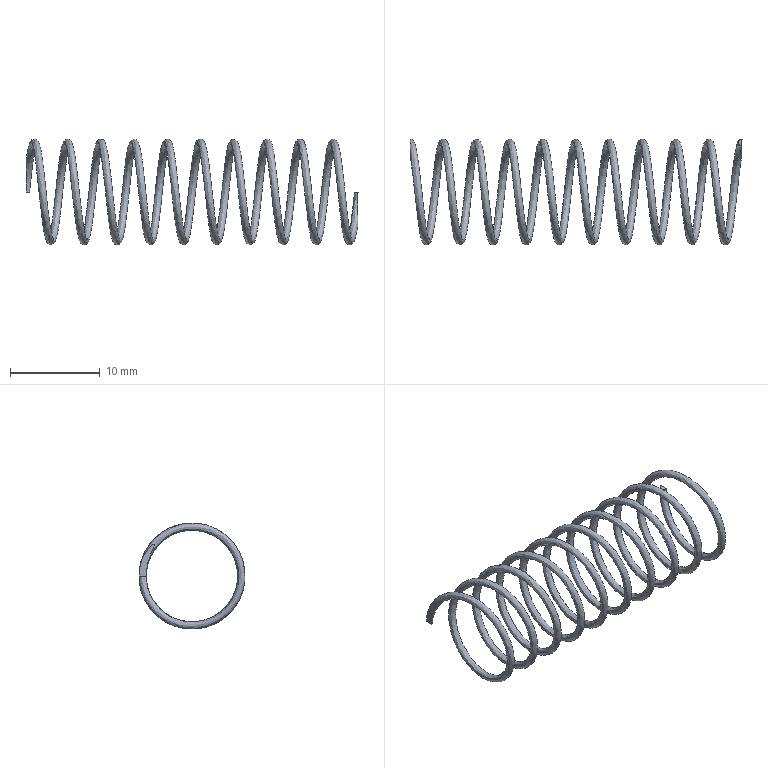Part | NX | features BREP 1, DATUM_CSYS 1 | 1 solid | 5 faces | box 37 x 11.8 x 11.8 mm | volume 173.342 mm3 | plane 4 | spline 1
STEP:
#1=CARTESIAN_POINT('',(0.,5.9,8.));
#2=VERTEX_POINT('',#1);
#3=CARTESIAN_POINT('',(0.,5.1,8.));
#4=VERTEX_POINT('',#3);
#5=CARTESIAN_POINT('',(0.,5.9,8.));
#6=DIRECTION('',(0.,-1.,0.));
#7=VECTOR('',#6,1000.);
#8=LINE('',#5,#7);
#9=EDGE_CURVE('',#2,#4,#8,.T.);
#10=ORIENTED_EDGE('',*,*,#9,.F.);
#11=CARTESIAN_POINT('',(0.4,5.5,8.));
#12=VERTEX_POINT('',#11);
#13=CARTESIAN_POINT('',(0.,5.5,8.));
#14=DIRECTION('',(0.,0.,-1.));
#15=DIRECTION('',(0.,1.,0.));
#16=AXIS2_PLACEMENT_3D('',#13,#14,#15);
#17=CIRCLE('',#16,0.4);
#18=EDGE_CURVE('',#2,#12,#17,.T.);
#19=ORIENTED_EDGE('',*,*,#18,.T.);
#20=CARTESIAN_POINT('',(0.,5.5,8.));
#21=DIRECTION('',(0.,0.,-1.));
#22=DIRECTION('',(1.,0.,0.));
#23=AXIS2_PLACEMENT_3D('',#20,#21,#22);
#24=CIRCLE('',#23,0.4);
#25=EDGE_CURVE('',#12,#4,#24,.T.);
#26=ORIENTED_EDGE('',*,*,#25,.T.);
#27=EDGE_LOOP('',(#10,#19,#26));
#28=FACE_BOUND('',#27,.T.);
#29=CARTESIAN_POINT('',(-0.2,5.5,8.));
#30=DIRECTION('',(0.,0.,1.));
#31=DIRECTION('',(0.,-1.,0.));
#32=AXIS2_PLACEMENT_3D('',#29,#30,#31);
#33=PLANE('',#32);
#34=ADVANCED_FACE('',(#28),#33,.F.);
#35=CARTESIAN_POINT('',(37.,4.228,4.482));
#36=VERTEX_POINT('',#35);
#37=CARTESIAN_POINT('',(0.4,5.5,8.));
#38=CARTESIAN_POINT('',(1.22,5.5,15.655));
#39=CARTESIAN_POINT('',(1.189,-1.995,17.212));
#40=CARTESIAN_POINT('',(2.009,-5.045,10.191));
#41=CARTESIAN_POINT('',(2.828,-8.094,3.17));
#42=CARTESIAN_POINT('',(2.798,-1.841,-1.245));
#43=CARTESIAN_POINT('',(3.617,3.754,3.98));
#44=CARTESIAN_POINT('',(4.437,9.349,9.205));
#45=CARTESIAN_POINT('',(4.406,5.371,15.746));
#46=CARTESIAN_POINT('',(5.226,-1.842,13.182));
#47=CARTESIAN_POINT('',(6.046,-9.055,10.619));
#48=CARTESIAN_POINT('',(6.015,-8.012,3.035));
#49=CARTESIAN_POINT('',(6.835,-0.3753,2.513));
#50=CARTESIAN_POINT('',(7.654,7.262,1.99));
#51=CARTESIAN_POINT('',(7.624,9.327,9.362));
#52=CARTESIAN_POINT('',(8.443,2.53,12.883));
#53=CARTESIAN_POINT('',(9.263,-4.266,16.405));
#54=CARTESIAN_POINT('',(9.233,-9.097,10.467));
#55=CARTESIAN_POINT('',(10.052,-4.266,4.529));
#56=CARTESIAN_POINT('',(10.872,0.5646,-1.409));
#57=CARTESIAN_POINT('',(10.841,7.361,2.113));
#58=CARTESIAN_POINT('',(11.661,5.296,9.484));
#59=CARTESIAN_POINT('',(12.48,3.231,16.855));
#60=CARTESIAN_POINT('',(12.45,-4.406,16.333));
#61=CARTESIAN_POINT('',(13.27,-5.449,8.749));
#62=CARTESIAN_POINT('',(14.089,-6.491,1.165));
#63=CARTESIAN_POINT('',(14.059,0.7219,-1.398));
#64=CARTESIAN_POINT('',(14.878,4.699,5.142));
#65=CARTESIAN_POINT('',(15.698,8.677,11.683));
#66=CARTESIAN_POINT('',(15.667,3.082,16.908));
#67=CARTESIAN_POINT('',(16.487,-3.172,12.493));
#68=CARTESIAN_POINT('',(17.307,-9.426,8.079));
#69=CARTESIAN_POINT('',(17.276,-6.376,1.058));
#70=CARTESIAN_POINT('',(18.096,1.119,2.615));
#71=CARTESIAN_POINT('',(18.915,8.614,4.172));
#72=CARTESIAN_POINT('',(18.885,8.614,11.828));
#73=CARTESIAN_POINT('',(19.704,1.119,13.385));
#74=CARTESIAN_POINT('',(20.524,-6.376,14.942));
#75=CARTESIAN_POINT('',(20.493,-9.426,7.921));
#76=CARTESIAN_POINT('',(21.313,-3.172,3.507));
#77=CARTESIAN_POINT('',(22.133,3.082,-0.9078));
#78=CARTESIAN_POINT('',(22.102,8.677,4.317));
#79=CARTESIAN_POINT('',(22.922,4.699,10.858));
#80=CARTESIAN_POINT('',(23.741,0.7219,17.398));
#81=CARTESIAN_POINT('',(23.711,-6.491,14.835));
#82=CARTESIAN_POINT('',(24.53,-5.449,7.251));
#83=CARTESIAN_POINT('',(25.35,-4.406,-0.3326));
#84=CARTESIAN_POINT('',(25.32,3.231,-0.855));
#85=CARTESIAN_POINT('',(26.139,5.296,6.516));
#86=CARTESIAN_POINT('',(26.959,7.361,13.887));
#87=CARTESIAN_POINT('',(26.928,0.5646,17.409));
#88=CARTESIAN_POINT('',(27.748,-4.266,11.471));
#89=CARTESIAN_POINT('',(28.567,-9.097,5.533));
#90=CARTESIAN_POINT('',(28.537,-4.266,-0.4052));
#91=CARTESIAN_POINT('',(29.357,2.53,3.117));
#92=CARTESIAN_POINT('',(30.176,9.327,6.638));
#93=CARTESIAN_POINT('',(30.146,7.262,14.01));
#94=CARTESIAN_POINT('',(30.965,-0.3753,13.487));
#95=CARTESIAN_POINT('',(31.785,-8.012,12.965));
#96=CARTESIAN_POINT('',(31.754,-9.055,5.381));
#97=CARTESIAN_POINT('',(32.574,-1.842,2.818));
#98=CARTESIAN_POINT('',(33.394,5.371,0.2541));
#99=CARTESIAN_POINT('',(33.363,9.349,6.795));
#100=CARTESIAN_POINT('',(34.183,3.754,12.02));
#101=CARTESIAN_POINT('',(35.002,-1.841,17.245));
#102=CARTESIAN_POINT('',(34.972,-8.094,12.83));
#103=CARTESIAN_POINT('',(35.791,-5.045,5.809));
#104=CARTESIAN_POINT('',(36.234,-3.397,2.017));
#105=CARTESIAN_POINT('',(36.466,1.025,0.6321));
#106=CARTESIAN_POINT('',(37.,4.228,4.482));
#107=(BOUNDED_CURVE()B_SPLINE_CURVE(3,(#37,#38,#39,#40,#41,#42,#43,#44,#45,#46,#47,#48,#49,#50,#51,#52,#53,#54,#55,#56,#57,#58,#59,#60,#61,#62,#63,#64,#65,#66,#67,#68,#69,#70,#71,#72,#73,#74,#75,#76,#77,#78,#79,#80,#81,#82,#83,#84,#85,#86,#87,#88,#89,#90,#91,#92,#93,#94,#95,#96,#97,#98,#99,#100,#101,#102,#103,#104,#105,#106),.UNSPECIFIED.,.F.,.F.)B_SPLINE_CURVE_WITH_KNOTS((4,3,3,3,3,3,3,3,3,3,3,3,3,3,3,3,3,3,3,3,3,3,3,4),(0.,0.04402,0.08805,0.1321,0.1761,0.2201,0.2641,0.3082,0.3522,0.3962,0.4402,0.4843,0.5283,0.5723,0.6163,0.6604,0.7044,0.7484,0.7924,0.8365,0.8805,0.9245,0.9685,1.),.PIECEWISE_BEZIER_KNOTS.)CURVE()GEOMETRIC_REPRESENTATION_ITEM()RATIONAL_B_SPLINE_CURVE((1.,0.469,0.469,1.,0.469,0.469,1.,0.469,0.469,1.,0.469,0.469,1.,0.469,0.469,1.,0.469,0.469,1.,0.469,0.469,1.,0.469,0.469,1.,0.469,0.469,1.,0.469,0.469,1.,0.469,0.469,1.,0.469,0.469,1.,0.469,0.469,1.,0.469,0.469,1.,0.469,0.469,1.,0.469,0.469,1.,0.469,0.469,1.,0.469,0.469,1.,0.469,0.469,1.,0.469,0.469,1.,0.469,0.469,1.,0.469,0.469,1.,0.6205,0.5122,0.6751))REPRESENTATION_ITEM(''));
#108=EDGE_CURVE('',#12,#36,#107,.T.);
#109=ORIENTED_EDGE('',*,*,#108,.T.);
#110=CARTESIAN_POINT('',(37.,5.1,8.));
#111=VERTEX_POINT('',#110);
#112=CARTESIAN_POINT('',(37.,5.1,8.));
#113=CARTESIAN_POINT('',(37.,5.1,7.692));
#114=CARTESIAN_POINT('',(37.,5.053,7.076));
#115=CARTESIAN_POINT('',(37.,4.883,6.333));
#116=CARTESIAN_POINT('',(37.,4.688,5.757));
#117=CARTESIAN_POINT('',(37.,4.521,5.335));
#118=CARTESIAN_POINT('',(37.,4.352,4.979));
#119=CARTESIAN_POINT('',(37.,4.255,4.714));
#120=CARTESIAN_POINT('',(37.,4.168,4.532));
#121=CARTESIAN_POINT('',(37.,4.228,4.482));
#122=B_SPLINE_CURVE_WITH_KNOTS('',3,(#112,#113,#114,#115,#116,#117,#118,#119,#120,#121),.UNSPECIFIED.,.F.,.F.,(4,1,1,1,1,1,1,4),(0.,0.0009216,0.001843,0.002304,0.002765,0.003226,0.003456,0.003686),.UNSPECIFIED.);
#123=EDGE_CURVE('',#111,#36,#122,.T.);
#124=ORIENTED_EDGE('',*,*,#123,.F.);
#125=CARTESIAN_POINT('',(37.,5.9,8.));
#126=VERTEX_POINT('',#125);
#127=CARTESIAN_POINT('',(37.,5.1,8.));
#128=CARTESIAN_POINT('',(36.893,5.1,8.));
#129=CARTESIAN_POINT('',(36.8,5.154,8.));
#130=CARTESIAN_POINT('',(36.2,5.5,8.));
#131=CARTESIAN_POINT('',(36.8,5.846,8.));
#132=CARTESIAN_POINT('',(36.893,5.9,8.));
#133=CARTESIAN_POINT('',(37.,5.9,8.));
#134=(BOUNDED_CURVE()B_SPLINE_CURVE(2,(#127,#128,#129,#130,#131,#132,#133),.UNSPECIFIED.,.F.,.F.)B_SPLINE_CURVE_WITH_KNOTS((3,2,2,3),(0.,0.1745,0.8255,1.),.PIECEWISE_BEZIER_KNOTS.)CURVE()GEOMETRIC_REPRESENTATION_ITEM()RATIONAL_B_SPLINE_CURVE((0.8038,0.866,1.,0.5,1.,0.866,0.8038))REPRESENTATION_ITEM(''));
#135=EDGE_CURVE('',#111,#126,#134,.T.);
#136=ORIENTED_EDGE('',*,*,#135,.T.);
#137=CARTESIAN_POINT('',(37.,4.228,4.482));
#138=CARTESIAN_POINT('',(37.,4.296,4.426));
#139=CARTESIAN_POINT('',(37.,4.477,4.579));
#140=CARTESIAN_POINT('',(37.,4.72,4.774));
#141=CARTESIAN_POINT('',(37.,5.005,5.12));
#142=CARTESIAN_POINT('',(37.,5.277,5.542));
#143=CARTESIAN_POINT('',(37.,5.582,6.162));
#144=CARTESIAN_POINT('',(37.,5.83,6.971));
#145=CARTESIAN_POINT('',(37.,5.9,7.657));
#146=CARTESIAN_POINT('',(37.,5.9,8.));
#147=B_SPLINE_CURVE_WITH_KNOTS('',3,(#137,#138,#139,#140,#141,#142,#143,#144,#145,#146),.UNSPECIFIED.,.F.,.F.,(4,1,1,1,1,1,1,4),(0.,0.0002623,0.0005247,0.001049,0.001574,0.002099,0.003148,0.004197),.UNSPECIFIED.);
#148=EDGE_CURVE('',#36,#126,#147,.T.);
#149=ORIENTED_EDGE('',*,*,#148,.F.);
#150=ORIENTED_EDGE('',*,*,#108,.F.);
#151=ORIENTED_EDGE('',*,*,#18,.F.);
#152=CARTESIAN_POINT('',(0.,5.1,8.));
#153=CARTESIAN_POINT('',(0.,5.1,8.329));
#154=CARTESIAN_POINT('',(0.,5.046,8.988));
#155=CARTESIAN_POINT('',(0.,4.815,9.94));
#156=CARTESIAN_POINT('',(0.,4.54,10.609));
#157=CARTESIAN_POINT('',(0.,4.34,11.07));
#158=CARTESIAN_POINT('',(0.,4.244,11.268));
#159=CARTESIAN_POINT('',(0.,4.173,11.609));
#160=CARTESIAN_POINT('',(0.,4.482,11.434));
#161=CARTESIAN_POINT('',(0.,4.64,11.288));
#162=CARTESIAN_POINT('',(0.,4.87,11.05));
#163=CARTESIAN_POINT('',(0.,5.106,10.734));
#164=CARTESIAN_POINT('',(0.,5.354,10.315));
#165=CARTESIAN_POINT('',(0.,5.617,9.735));
#166=CARTESIAN_POINT('',(0.,5.84,8.964));
#167=CARTESIAN_POINT('',(0.,5.9,8.322));
#168=CARTESIAN_POINT('',(0.,5.9,8.));
#169=B_SPLINE_CURVE_WITH_KNOTS('',3,(#152,#153,#154,#155,#156,#157,#158,#159,#160,#161,#162,#163,#164,#165,#166,#167,#168),.UNSPECIFIED.,.F.,.F.,(4,1,1,1,1,1,1,1,1,1,1,1,1,1,4),(0.,0.0009854,0.001971,0.002956,0.003203,0.003449,0.003695,0.003942,0.004188,0.004434,0.004927,0.00542,0.005912,0.006898,0.007883),.UNSPECIFIED.);
#170=EDGE_CURVE('',#4,#2,#169,.T.);
#171=ORIENTED_EDGE('',*,*,#170,.F.);
#172=ORIENTED_EDGE('',*,*,#25,.F.);
#173=EDGE_LOOP('',(#109,#124,#136,#149,#150,#151,#171,#172));
#174=FACE_BOUND('',#173,.T.);
#175=CARTESIAN_POINT('',(0.4,5.5,8.));
#176=CARTESIAN_POINT('',(1.22,5.5,15.655));
#177=CARTESIAN_POINT('',(1.189,-1.995,17.212));
#178=CARTESIAN_POINT('',(2.009,-5.045,10.191));
#179=CARTESIAN_POINT('',(2.828,-8.094,3.17));
#180=CARTESIAN_POINT('',(2.798,-1.841,-1.245));
#181=CARTESIAN_POINT('',(3.617,3.754,3.98));
#182=CARTESIAN_POINT('',(4.437,9.349,9.205));
#183=CARTESIAN_POINT('',(4.406,5.371,15.746));
#184=CARTESIAN_POINT('',(5.226,-1.842,13.182));
#185=CARTESIAN_POINT('',(6.046,-9.055,10.619));
#186=CARTESIAN_POINT('',(6.015,-8.012,3.035));
#187=CARTESIAN_POINT('',(6.835,-0.3753,2.513));
#188=CARTESIAN_POINT('',(7.654,7.262,1.99));
#189=CARTESIAN_POINT('',(7.624,9.327,9.362));
#190=CARTESIAN_POINT('',(8.443,2.53,12.883));
#191=CARTESIAN_POINT('',(9.263,-4.266,16.405));
#192=CARTESIAN_POINT('',(9.233,-9.097,10.467));
#193=CARTESIAN_POINT('',(10.052,-4.266,4.529));
#194=CARTESIAN_POINT('',(10.872,0.5646,-1.409));
#195=CARTESIAN_POINT('',(10.841,7.361,2.113));
#196=CARTESIAN_POINT('',(11.661,5.296,9.484));
#197=CARTESIAN_POINT('',(12.48,3.231,16.855));
#198=CARTESIAN_POINT('',(12.45,-4.406,16.333));
#199=CARTESIAN_POINT('',(13.27,-5.449,8.749));
#200=CARTESIAN_POINT('',(14.089,-6.491,1.165));
#201=CARTESIAN_POINT('',(14.059,0.7219,-1.398));
#202=CARTESIAN_POINT('',(14.878,4.699,5.142));
#203=CARTESIAN_POINT('',(15.698,8.677,11.683));
#204=CARTESIAN_POINT('',(15.667,3.082,16.908));
#205=CARTESIAN_POINT('',(16.487,-3.172,12.493));
#206=CARTESIAN_POINT('',(17.307,-9.426,8.079));
#207=CARTESIAN_POINT('',(17.276,-6.376,1.058));
#208=CARTESIAN_POINT('',(18.096,1.119,2.615));
#209=CARTESIAN_POINT('',(18.915,8.614,4.172));
#210=CARTESIAN_POINT('',(18.885,8.614,11.828));
#211=CARTESIAN_POINT('',(19.704,1.119,13.385));
#212=CARTESIAN_POINT('',(20.524,-6.376,14.942));
#213=CARTESIAN_POINT('',(20.493,-9.426,7.921));
#214=CARTESIAN_POINT('',(21.313,-3.172,3.507));
#215=CARTESIAN_POINT('',(22.133,3.082,-0.9078));
#216=CARTESIAN_POINT('',(22.102,8.677,4.317));
#217=CARTESIAN_POINT('',(22.922,4.699,10.858));
#218=CARTESIAN_POINT('',(23.741,0.7219,17.398));
#219=CARTESIAN_POINT('',(23.711,-6.491,14.835));
#220=CARTESIAN_POINT('',(24.53,-5.449,7.251));
#221=CARTESIAN_POINT('',(25.35,-4.406,-0.3326));
#222=CARTESIAN_POINT('',(25.32,3.231,-0.855));
#223=CARTESIAN_POINT('',(26.139,5.296,6.516));
#224=CARTESIAN_POINT('',(26.959,7.361,13.887));
#225=CARTESIAN_POINT('',(26.928,0.5646,17.409));
#226=CARTESIAN_POINT('',(27.748,-4.266,11.471));
#227=CARTESIAN_POINT('',(28.567,-9.097,5.533));
#228=CARTESIAN_POINT('',(28.537,-4.266,-0.4052));
#229=CARTESIAN_POINT('',(29.357,2.53,3.117));
#230=CARTESIAN_POINT('',(30.176,9.327,6.638));
#231=CARTESIAN_POINT('',(30.146,7.262,14.01));
#232=CARTESIAN_POINT('',(30.965,-0.3753,13.487));
#233=CARTESIAN_POINT('',(31.785,-8.012,12.965));
#234=CARTESIAN_POINT('',(31.754,-9.055,5.381));
#235=CARTESIAN_POINT('',(32.574,-1.842,2.818));
#236=CARTESIAN_POINT('',(33.394,5.371,0.2541));
#237=CARTESIAN_POINT('',(33.363,9.349,6.795));
#238=CARTESIAN_POINT('',(34.183,3.754,12.02));
#239=CARTESIAN_POINT('',(35.002,-1.841,17.245));
#240=CARTESIAN_POINT('',(34.972,-8.094,12.83));
#241=CARTESIAN_POINT('',(35.791,-5.045,5.809));
#242=CARTESIAN_POINT('',(36.611,-1.995,-1.212));
#243=CARTESIAN_POINT('',(36.58,5.5,0.345));
#244=CARTESIAN_POINT('',(37.4,5.5,8.));
#245=CARTESIAN_POINT('',(0.4,4.807,8.));
#246=CARTESIAN_POINT('',(1.22,4.807,14.691));
#247=CARTESIAN_POINT('',(1.189,-1.744,16.052));
#248=CARTESIAN_POINT('',(2.009,-4.409,9.915));
#249=CARTESIAN_POINT('',(2.828,-7.075,3.778));
#250=CARTESIAN_POINT('',(2.798,-1.609,-0.08004));
#251=CARTESIAN_POINT('',(3.617,3.281,4.487));
#252=CARTESIAN_POINT('',(4.437,8.171,9.054));
#253=CARTESIAN_POINT('',(4.406,4.695,14.77));
#254=CARTESIAN_POINT('',(5.226,-1.61,12.53));
#255=CARTESIAN_POINT('',(6.046,-7.914,10.289));
#256=CARTESIAN_POINT('',(6.015,-7.003,3.661));
#257=CARTESIAN_POINT('',(6.835,-0.3281,3.204));
#258=CARTESIAN_POINT('',(7.654,6.347,2.747));
#259=CARTESIAN_POINT('',(7.624,8.152,9.19));
#260=CARTESIAN_POINT('',(8.443,2.212,12.268));
#261=CARTESIAN_POINT('',(9.263,-3.729,15.346));
#262=CARTESIAN_POINT('',(9.233,-7.951,10.156));
#263=CARTESIAN_POINT('',(10.052,-3.729,4.966));
#264=CARTESIAN_POINT('',(10.872,0.4935,-0.2238));
#265=CARTESIAN_POINT('',(10.841,6.434,2.854));
#266=CARTESIAN_POINT('',(11.661,4.629,9.297));
#267=CARTESIAN_POINT('',(12.48,2.824,15.74));
#268=CARTESIAN_POINT('',(12.45,-3.851,15.283));
#269=CARTESIAN_POINT('',(13.27,-4.762,8.655));
#270=CARTESIAN_POINT('',(14.089,-5.673,2.026));
#271=CARTESIAN_POINT('',(14.059,0.631,-0.2144));
#272=CARTESIAN_POINT('',(14.878,4.107,5.502));
#273=CARTESIAN_POINT('',(15.698,7.584,11.219));
#274=CARTESIAN_POINT('',(15.667,2.694,15.786));
#275=CARTESIAN_POINT('',(16.487,-2.772,11.927));
#276=CARTESIAN_POINT('',(17.307,-8.238,8.069));
#277=CARTESIAN_POINT('',(17.276,-5.573,1.932));
#278=CARTESIAN_POINT('',(18.096,0.978,3.293));
#279=CARTESIAN_POINT('',(18.915,7.529,4.655));
#280=CARTESIAN_POINT('',(18.885,7.529,11.345));
#281=CARTESIAN_POINT('',(19.704,0.978,12.707));
#282=CARTESIAN_POINT('',(20.524,-5.573,14.068));
#283=CARTESIAN_POINT('',(20.493,-8.238,7.931));
#284=CARTESIAN_POINT('',(21.313,-2.772,4.073));
#285=CARTESIAN_POINT('',(22.133,2.694,0.2143));
#286=CARTESIAN_POINT('',(22.102,7.584,4.781));
#287=CARTESIAN_POINT('',(22.922,4.107,10.498));
#288=CARTESIAN_POINT('',(23.741,0.631,16.214));
#289=CARTESIAN_POINT('',(23.711,-5.673,13.974));
#290=CARTESIAN_POINT('',(24.53,-4.762,7.345));
#291=CARTESIAN_POINT('',(25.35,-3.851,0.717));
#292=CARTESIAN_POINT('',(25.32,2.824,0.2604));
#293=CARTESIAN_POINT('',(26.139,4.629,6.703));
#294=CARTESIAN_POINT('',(26.959,6.434,13.146));
#295=CARTESIAN_POINT('',(26.928,0.4935,16.224));
#296=CARTESIAN_POINT('',(27.748,-3.729,11.034));
#297=CARTESIAN_POINT('',(28.567,-7.951,5.844));
#298=CARTESIAN_POINT('',(28.537,-3.729,0.6536));
#299=CARTESIAN_POINT('',(29.357,2.212,3.732));
#300=CARTESIAN_POINT('',(30.176,8.152,6.81));
#301=CARTESIAN_POINT('',(30.146,6.347,13.253));
#302=CARTESIAN_POINT('',(30.965,-0.3281,12.796));
#303=CARTESIAN_POINT('',(31.785,-7.003,12.339));
#304=CARTESIAN_POINT('',(31.754,-7.914,5.711));
#305=CARTESIAN_POINT('',(32.574,-1.61,3.47));
#306=CARTESIAN_POINT('',(33.394,4.695,1.23));
#307=CARTESIAN_POINT('',(33.363,8.171,6.946));
#308=CARTESIAN_POINT('',(34.183,3.281,11.513));
#309=CARTESIAN_POINT('',(35.002,-1.609,16.08));
#310=CARTESIAN_POINT('',(34.972,-7.075,12.222));
#311=CARTESIAN_POINT('',(35.791,-4.409,6.085));
#312=CARTESIAN_POINT('',(36.611,-1.744,-0.052));
#313=CARTESIAN_POINT('',(36.58,4.807,1.309));
#314=CARTESIAN_POINT('',(37.4,4.807,8.));
#315=CARTESIAN_POINT('',(-0.2,5.154,8.));
#316=CARTESIAN_POINT('',(0.6196,5.154,15.173));
#317=CARTESIAN_POINT('',(0.5891,-1.869,16.632));
#318=CARTESIAN_POINT('',(1.409,-4.727,10.053));
#319=CARTESIAN_POINT('',(2.228,-7.585,3.474));
#320=CARTESIAN_POINT('',(2.198,-1.725,-0.6623));
#321=CARTESIAN_POINT('',(3.017,3.518,4.234));
#322=CARTESIAN_POINT('',(3.837,8.76,9.129));
#323=CARTESIAN_POINT('',(3.806,5.033,15.258));
#324=CARTESIAN_POINT('',(4.626,-1.726,12.856));
#325=CARTESIAN_POINT('',(5.446,-8.485,10.454));
#326=CARTESIAN_POINT('',(5.415,-7.508,3.348));
#327=CARTESIAN_POINT('',(6.235,-0.3517,2.858));
#328=CARTESIAN_POINT('',(7.054,6.804,2.369));
#329=CARTESIAN_POINT('',(7.024,8.74,9.276));
#330=CARTESIAN_POINT('',(7.843,2.371,12.576));
#331=CARTESIAN_POINT('',(8.663,-3.998,15.876));
#332=CARTESIAN_POINT('',(8.633,-8.524,10.312));
#333=CARTESIAN_POINT('',(9.452,-3.998,4.748));
#334=CARTESIAN_POINT('',(10.272,0.529,-0.8164));
#335=CARTESIAN_POINT('',(10.241,6.898,2.484));
#336=CARTESIAN_POINT('',(11.061,4.962,9.39));
#337=CARTESIAN_POINT('',(11.88,3.027,16.297));
#338=CARTESIAN_POINT('',(11.85,-4.129,15.808));
#339=CARTESIAN_POINT('',(12.67,-5.106,8.702));
#340=CARTESIAN_POINT('',(13.489,-6.082,1.596));
#341=CARTESIAN_POINT('',(13.459,0.6764,-0.8064));
#342=CARTESIAN_POINT('',(14.278,4.403,5.322));
#343=CARTESIAN_POINT('',(15.098,8.13,11.451));
#344=CARTESIAN_POINT('',(15.067,2.888,16.347));
#345=CARTESIAN_POINT('',(15.887,-2.972,12.21));
#346=CARTESIAN_POINT('',(16.707,-8.832,8.074));
#347=CARTESIAN_POINT('',(16.676,-5.974,1.495));
#348=CARTESIAN_POINT('',(17.496,1.049,2.954));
#349=CARTESIAN_POINT('',(18.315,8.071,4.414));
#350=CARTESIAN_POINT('',(18.285,8.071,11.586));
#351=CARTESIAN_POINT('',(19.104,1.049,13.046));
#352=CARTESIAN_POINT('',(19.924,-5.974,14.505));
#353=CARTESIAN_POINT('',(19.893,-8.832,7.926));
#354=CARTESIAN_POINT('',(20.713,-2.972,3.79));
#355=CARTESIAN_POINT('',(21.533,2.888,-0.3468));
#356=CARTESIAN_POINT('',(21.502,8.13,4.549));
#357=CARTESIAN_POINT('',(22.322,4.403,10.678));
#358=CARTESIAN_POINT('',(23.141,0.6764,16.806));
#359=CARTESIAN_POINT('',(23.111,-6.082,14.404));
#360=CARTESIAN_POINT('',(23.93,-5.106,7.298));
#361=CARTESIAN_POINT('',(24.75,-4.129,0.1922));
#362=CARTESIAN_POINT('',(24.72,3.027,-0.2973));
#363=CARTESIAN_POINT('',(25.539,4.962,6.61));
#364=CARTESIAN_POINT('',(26.359,6.898,13.516));
#365=CARTESIAN_POINT('',(26.328,0.529,16.816));
#366=CARTESIAN_POINT('',(27.148,-3.998,11.252));
#367=CARTESIAN_POINT('',(27.967,-8.524,5.688));
#368=CARTESIAN_POINT('',(27.937,-3.998,0.1242));
#369=CARTESIAN_POINT('',(28.757,2.371,3.424));
#370=CARTESIAN_POINT('',(29.576,8.74,6.724));
#371=CARTESIAN_POINT('',(29.546,6.804,13.631));
#372=CARTESIAN_POINT('',(30.365,-0.3517,13.142));
#373=CARTESIAN_POINT('',(31.185,-7.508,12.652));
#374=CARTESIAN_POINT('',(31.154,-8.485,5.546));
#375=CARTESIAN_POINT('',(31.974,-1.726,3.144));
#376=CARTESIAN_POINT('',(32.794,5.033,0.7419));
#377=CARTESIAN_POINT('',(32.763,8.76,6.871));
#378=CARTESIAN_POINT('',(33.583,3.518,11.766));
#379=CARTESIAN_POINT('',(34.402,-1.725,16.662));
#380=CARTESIAN_POINT('',(34.372,-7.585,12.526));
#381=CARTESIAN_POINT('',(35.191,-4.727,5.947));
#382=CARTESIAN_POINT('',(36.011,-1.869,-0.6322));
#383=CARTESIAN_POINT('',(35.98,5.154,0.8271));
#384=CARTESIAN_POINT('',(36.8,5.154,8.));
#385=CARTESIAN_POINT('',(-0.8,5.5,8.));
#386=CARTESIAN_POINT('',(0.01961,5.5,15.655));
#387=CARTESIAN_POINT('',(-0.01091,-1.995,17.212));
#388=CARTESIAN_POINT('',(0.8087,-5.045,10.191));
#389=CARTESIAN_POINT('',(1.628,-8.094,3.17));
#390=CARTESIAN_POINT('',(1.598,-1.841,-1.245));
#391=CARTESIAN_POINT('',(2.417,3.754,3.98));
#392=CARTESIAN_POINT('',(3.237,9.349,9.205));
#393=CARTESIAN_POINT('',(3.206,5.371,15.746));
#394=CARTESIAN_POINT('',(4.026,-1.842,13.182));
#395=CARTESIAN_POINT('',(4.846,-9.055,10.619));
#396=CARTESIAN_POINT('',(4.815,-8.012,3.035));
#397=CARTESIAN_POINT('',(5.635,-0.3753,2.513));
#398=CARTESIAN_POINT('',(6.454,7.262,1.99));
#399=CARTESIAN_POINT('',(6.424,9.327,9.362));
#400=CARTESIAN_POINT('',(7.243,2.53,12.883));
#401=CARTESIAN_POINT('',(8.063,-4.266,16.405));
#402=CARTESIAN_POINT('',(8.033,-9.097,10.467));
#403=CARTESIAN_POINT('',(8.852,-4.266,4.529));
#404=CARTESIAN_POINT('',(9.672,0.5646,-1.409));
#405=CARTESIAN_POINT('',(9.641,7.361,2.113));
#406=CARTESIAN_POINT('',(10.461,5.296,9.484));
#407=CARTESIAN_POINT('',(11.28,3.231,16.855));
#408=CARTESIAN_POINT('',(11.25,-4.406,16.333));
#409=CARTESIAN_POINT('',(12.07,-5.449,8.749));
#410=CARTESIAN_POINT('',(12.889,-6.491,1.165));
#411=CARTESIAN_POINT('',(12.859,0.7219,-1.398));
#412=CARTESIAN_POINT('',(13.678,4.699,5.142));
#413=CARTESIAN_POINT('',(14.498,8.677,11.683));
#414=CARTESIAN_POINT('',(14.467,3.082,16.908));
#415=CARTESIAN_POINT('',(15.287,-3.172,12.493));
#416=CARTESIAN_POINT('',(16.107,-9.426,8.079));
#417=CARTESIAN_POINT('',(16.076,-6.376,1.058));
#418=CARTESIAN_POINT('',(16.896,1.119,2.615));
#419=CARTESIAN_POINT('',(17.715,8.614,4.172));
#420=CARTESIAN_POINT('',(17.685,8.614,11.828));
#421=CARTESIAN_POINT('',(18.504,1.119,13.385));
#422=CARTESIAN_POINT('',(19.324,-6.376,14.942));
#423=CARTESIAN_POINT('',(19.293,-9.426,7.921));
#424=CARTESIAN_POINT('',(20.113,-3.172,3.507));
#425=CARTESIAN_POINT('',(20.933,3.082,-0.9078));
#426=CARTESIAN_POINT('',(20.902,8.677,4.317));
#427=CARTESIAN_POINT('',(21.722,4.699,10.858));
#428=CARTESIAN_POINT('',(22.541,0.7219,17.398));
#429=CARTESIAN_POINT('',(22.511,-6.491,14.835));
#430=CARTESIAN_POINT('',(23.33,-5.449,7.251));
#431=CARTESIAN_POINT('',(24.15,-4.406,-0.3326));
#432=CARTESIAN_POINT('',(24.12,3.231,-0.855));
#433=CARTESIAN_POINT('',(24.939,5.296,6.516));
#434=CARTESIAN_POINT('',(25.759,7.361,13.887));
#435=CARTESIAN_POINT('',(25.728,0.5646,17.409));
#436=CARTESIAN_POINT('',(26.548,-4.266,11.471));
#437=CARTESIAN_POINT('',(27.367,-9.097,5.533));
#438=CARTESIAN_POINT('',(27.337,-4.266,-0.4052));
#439=CARTESIAN_POINT('',(28.157,2.53,3.117));
#440=CARTESIAN_POINT('',(28.976,9.327,6.638));
#441=CARTESIAN_POINT('',(28.946,7.262,14.01));
#442=CARTESIAN_POINT('',(29.765,-0.3753,13.487));
#443=CARTESIAN_POINT('',(30.585,-8.012,12.965));
#444=CARTESIAN_POINT('',(30.554,-9.055,5.381));
#445=CARTESIAN_POINT('',(31.374,-1.842,2.818));
#446=CARTESIAN_POINT('',(32.194,5.371,0.2541));
#447=CARTESIAN_POINT('',(32.163,9.349,6.795));
#448=CARTESIAN_POINT('',(32.983,3.754,12.02));
#449=CARTESIAN_POINT('',(33.802,-1.841,17.245));
#450=CARTESIAN_POINT('',(33.772,-8.094,12.83));
#451=CARTESIAN_POINT('',(34.591,-5.045,5.809));
#452=CARTESIAN_POINT('',(35.411,-1.995,-1.212));
#453=CARTESIAN_POINT('',(35.38,5.5,0.345));
#454=CARTESIAN_POINT('',(36.2,5.5,8.));
#455=CARTESIAN_POINT('',(-0.2,5.846,8.));
#456=CARTESIAN_POINT('',(0.6196,5.846,16.137));
#457=CARTESIAN_POINT('',(0.5891,-2.121,17.793));
#458=CARTESIAN_POINT('',(1.409,-5.362,10.329));
#459=CARTESIAN_POINT('',(2.228,-8.604,2.866));
#460=CARTESIAN_POINT('',(2.198,-1.956,-1.827));
#461=CARTESIAN_POINT('',(3.017,3.99,3.727));
#462=CARTESIAN_POINT('',(3.837,9.937,9.281));
#463=CARTESIAN_POINT('',(3.806,5.709,16.234));
#464=CARTESIAN_POINT('',(4.626,-1.958,13.509));
#465=CARTESIAN_POINT('',(5.446,-9.625,10.784));
#466=CARTESIAN_POINT('',(5.415,-8.517,2.723));
#467=CARTESIAN_POINT('',(6.235,-0.399,2.167));
#468=CARTESIAN_POINT('',(7.054,7.719,1.612));
#469=CARTESIAN_POINT('',(7.024,9.915,9.447));
#470=CARTESIAN_POINT('',(7.843,2.69,13.191));
#471=CARTESIAN_POINT('',(8.663,-4.535,16.935));
#472=CARTESIAN_POINT('',(8.633,-9.67,10.622));
#473=CARTESIAN_POINT('',(9.452,-4.535,4.31));
#474=CARTESIAN_POINT('',(10.272,0.6001,-2.002));
#475=CARTESIAN_POINT('',(10.241,7.825,1.742));
#476=CARTESIAN_POINT('',(11.061,5.63,9.577));
#477=CARTESIAN_POINT('',(11.88,3.434,17.413));
#478=CARTESIAN_POINT('',(11.85,-4.684,16.857));
#479=CARTESIAN_POINT('',(12.67,-5.792,8.796));
#480=CARTESIAN_POINT('',(13.489,-6.9,0.7347));
#481=CARTESIAN_POINT('',(13.459,0.7674,-1.99));
#482=CARTESIAN_POINT('',(14.278,4.995,4.962));
#483=CARTESIAN_POINT('',(15.098,9.223,11.915));
#484=CARTESIAN_POINT('',(15.067,3.276,17.469));
#485=CARTESIAN_POINT('',(15.887,-3.372,12.776));
#486=CARTESIAN_POINT('',(16.707,-10.019,8.084));
#487=CARTESIAN_POINT('',(16.676,-6.777,0.6203));
#488=CARTESIAN_POINT('',(17.496,1.189,2.276));
#489=CARTESIAN_POINT('',(18.315,9.156,3.931));
#490=CARTESIAN_POINT('',(18.285,9.156,12.069));
#491=CARTESIAN_POINT('',(19.104,1.189,13.724));
#492=CARTESIAN_POINT('',(19.924,-6.777,15.38));
#493=CARTESIAN_POINT('',(19.893,-10.019,7.916));
#494=CARTESIAN_POINT('',(20.713,-3.372,3.224));
#495=CARTESIAN_POINT('',(21.533,3.276,-1.469));
#496=CARTESIAN_POINT('',(21.502,9.223,4.085));
#497=CARTESIAN_POINT('',(22.322,4.995,11.038));
#498=CARTESIAN_POINT('',(23.141,0.7674,17.99));
#499=CARTESIAN_POINT('',(23.111,-6.9,15.265));
#500=CARTESIAN_POINT('',(23.93,-5.792,7.204));
#501=CARTESIAN_POINT('',(24.75,-4.684,-0.8574));
#502=CARTESIAN_POINT('',(24.72,3.434,-1.413));
#503=CARTESIAN_POINT('',(25.539,5.63,6.423));
#504=CARTESIAN_POINT('',(26.359,7.825,14.258));
#505=CARTESIAN_POINT('',(26.328,0.6001,18.002));
#506=CARTESIAN_POINT('',(27.148,-4.535,11.69));
#507=CARTESIAN_POINT('',(27.967,-9.67,5.378));
#508=CARTESIAN_POINT('',(27.937,-4.535,-0.9346));
#509=CARTESIAN_POINT('',(28.757,2.69,2.809));
#510=CARTESIAN_POINT('',(29.576,9.915,6.553));
#511=CARTESIAN_POINT('',(29.546,7.719,14.388));
#512=CARTESIAN_POINT('',(30.365,-0.399,13.833));
#513=CARTESIAN_POINT('',(31.185,-8.517,13.277));
#514=CARTESIAN_POINT('',(31.154,-9.625,5.216));
#515=CARTESIAN_POINT('',(31.974,-1.958,2.491));
#516=CARTESIAN_POINT('',(32.794,5.709,-0.2338));
#517=CARTESIAN_POINT('',(32.763,9.937,6.719));
#518=CARTESIAN_POINT('',(33.583,3.99,12.273));
#519=CARTESIAN_POINT('',(34.402,-1.956,17.827));
#520=CARTESIAN_POINT('',(34.372,-8.604,13.134));
#521=CARTESIAN_POINT('',(35.191,-5.362,5.671));
#522=CARTESIAN_POINT('',(36.011,-2.121,-1.793));
#523=CARTESIAN_POINT('',(35.98,5.846,-0.1372));
#524=CARTESIAN_POINT('',(36.8,5.846,8.));
#525=CARTESIAN_POINT('',(0.4,6.193,8.));
#526=CARTESIAN_POINT('',(1.22,6.193,16.619));
#527=CARTESIAN_POINT('',(1.189,-2.246,18.373));
#528=CARTESIAN_POINT('',(2.009,-5.68,10.467));
#529=CARTESIAN_POINT('',(2.828,-9.114,2.562));
#530=CARTESIAN_POINT('',(2.798,-2.072,-2.409));
#531=CARTESIAN_POINT('',(3.617,4.227,3.474));
#532=CARTESIAN_POINT('',(4.437,10.526,9.357));
#533=CARTESIAN_POINT('',(4.406,6.048,16.722));
#534=CARTESIAN_POINT('',(5.226,-2.074,13.835));
#535=CARTESIAN_POINT('',(6.046,-10.195,10.949));
#536=CARTESIAN_POINT('',(6.015,-9.022,2.41));
#537=CARTESIAN_POINT('',(6.835,-0.4226,1.822));
#538=CARTESIAN_POINT('',(7.654,8.177,1.233));
#539=CARTESIAN_POINT('',(7.624,10.502,9.533));
#540=CARTESIAN_POINT('',(8.443,2.849,13.499));
#541=CARTESIAN_POINT('',(9.263,-4.804,17.464));
#542=CARTESIAN_POINT('',(9.233,-10.243,10.778));
#543=CARTESIAN_POINT('',(10.052,-4.804,4.092));
#544=CARTESIAN_POINT('',(10.872,0.6357,-2.594));
#545=CARTESIAN_POINT('',(10.841,8.289,1.371));
#546=CARTESIAN_POINT('',(11.661,5.963,9.671));
#547=CARTESIAN_POINT('',(12.48,3.638,17.97));
#548=CARTESIAN_POINT('',(12.45,-4.961,17.382));
#549=CARTESIAN_POINT('',(13.27,-6.135,8.843));
#550=CARTESIAN_POINT('',(14.089,-7.309,0.3042));
#551=CARTESIAN_POINT('',(14.059,0.8128,-2.582));
#552=CARTESIAN_POINT('',(14.878,5.291,4.782));
#553=CARTESIAN_POINT('',(15.698,9.77,12.147));
#554=CARTESIAN_POINT('',(15.667,3.47,18.03));
#555=CARTESIAN_POINT('',(16.487,-3.571,13.059));
#556=CARTESIAN_POINT('',(17.307,-10.613,8.089));
#557=CARTESIAN_POINT('',(17.276,-7.179,0.1831));
#558=CARTESIAN_POINT('',(18.096,1.26,1.937));
#559=CARTESIAN_POINT('',(18.915,9.699,3.69));
#560=CARTESIAN_POINT('',(18.885,9.699,12.31));
#561=CARTESIAN_POINT('',(19.704,1.26,14.063));
#562=CARTESIAN_POINT('',(20.524,-7.179,15.817));
#563=CARTESIAN_POINT('',(20.493,-10.613,7.911));
#564=CARTESIAN_POINT('',(21.313,-3.571,2.941));
#565=CARTESIAN_POINT('',(22.133,3.47,-2.03));
#566=CARTESIAN_POINT('',(22.102,9.77,3.853));
#567=CARTESIAN_POINT('',(22.922,5.291,11.218));
#568=CARTESIAN_POINT('',(23.741,0.8128,18.582));
#569=CARTESIAN_POINT('',(23.711,-7.309,15.696));
#570=CARTESIAN_POINT('',(24.53,-6.135,7.157));
#571=CARTESIAN_POINT('',(25.35,-4.961,-1.382));
#572=CARTESIAN_POINT('',(25.32,3.638,-1.97));
#573=CARTESIAN_POINT('',(26.139,5.963,6.329));
#574=CARTESIAN_POINT('',(26.959,8.289,14.629));
#575=CARTESIAN_POINT('',(26.928,0.6357,18.594));
#576=CARTESIAN_POINT('',(27.748,-4.804,11.908));
#577=CARTESIAN_POINT('',(28.567,-10.243,5.222));
#578=CARTESIAN_POINT('',(28.537,-4.804,-1.464));
#579=CARTESIAN_POINT('',(29.357,2.849,2.501));
#580=CARTESIAN_POINT('',(30.176,10.502,6.467));
#581=CARTESIAN_POINT('',(30.146,8.177,14.767));
#582=CARTESIAN_POINT('',(30.965,-0.4226,14.178));
#583=CARTESIAN_POINT('',(31.785,-9.022,13.59));
#584=CARTESIAN_POINT('',(31.754,-10.195,5.051));
#585=CARTESIAN_POINT('',(32.574,-2.074,2.165));
#586=CARTESIAN_POINT('',(33.394,6.048,-0.7217));
#587=CARTESIAN_POINT('',(33.363,10.526,6.643));
#588=CARTESIAN_POINT('',(34.183,4.227,12.526));
#589=CARTESIAN_POINT('',(35.002,-2.072,18.409));
#590=CARTESIAN_POINT('',(34.972,-9.114,13.438));
#591=CARTESIAN_POINT('',(35.791,-5.68,5.533));
#592=CARTESIAN_POINT('',(36.611,-2.246,-2.373));
#593=CARTESIAN_POINT('',(36.58,6.193,-0.6193));
#594=CARTESIAN_POINT('',(37.4,6.193,8.));
#595=CARTESIAN_POINT('',(0.4,5.5,8.));
#596=CARTESIAN_POINT('',(1.22,5.5,15.655));
#597=CARTESIAN_POINT('',(1.189,-1.995,17.212));
#598=CARTESIAN_POINT('',(2.009,-5.045,10.191));
#599=CARTESIAN_POINT('',(2.828,-8.094,3.17));
#600=CARTESIAN_POINT('',(2.798,-1.841,-1.245));
#601=CARTESIAN_POINT('',(3.617,3.754,3.98));
#602=CARTESIAN_POINT('',(4.437,9.349,9.205));
#603=CARTESIAN_POINT('',(4.406,5.371,15.746));
#604=CARTESIAN_POINT('',(5.226,-1.842,13.182));
#605=CARTESIAN_POINT('',(6.046,-9.055,10.619));
#606=CARTESIAN_POINT('',(6.015,-8.012,3.035));
#607=CARTESIAN_POINT('',(6.835,-0.3753,2.513));
#608=CARTESIAN_POINT('',(7.654,7.262,1.99));
#609=CARTESIAN_POINT('',(7.624,9.327,9.362));
#610=CARTESIAN_POINT('',(8.443,2.53,12.883));
#611=CARTESIAN_POINT('',(9.263,-4.266,16.405));
#612=CARTESIAN_POINT('',(9.233,-9.097,10.467));
#613=CARTESIAN_POINT('',(10.052,-4.266,4.529));
#614=CARTESIAN_POINT('',(10.872,0.5646,-1.409));
#615=CARTESIAN_POINT('',(10.841,7.361,2.113));
#616=CARTESIAN_POINT('',(11.661,5.296,9.484));
#617=CARTESIAN_POINT('',(12.48,3.231,16.855));
#618=CARTESIAN_POINT('',(12.45,-4.406,16.333));
#619=CARTESIAN_POINT('',(13.27,-5.449,8.749));
#620=CARTESIAN_POINT('',(14.089,-6.491,1.165));
#621=CARTESIAN_POINT('',(14.059,0.7219,-1.398));
#622=CARTESIAN_POINT('',(14.878,4.699,5.142));
#623=CARTESIAN_POINT('',(15.698,8.677,11.683));
#624=CARTESIAN_POINT('',(15.667,3.082,16.908));
#625=CARTESIAN_POINT('',(16.487,-3.172,12.493));
#626=CARTESIAN_POINT('',(17.307,-9.426,8.079));
#627=CARTESIAN_POINT('',(17.276,-6.376,1.058));
#628=CARTESIAN_POINT('',(18.096,1.119,2.615));
#629=CARTESIAN_POINT('',(18.915,8.614,4.172));
#630=CARTESIAN_POINT('',(18.885,8.614,11.828));
#631=CARTESIAN_POINT('',(19.704,1.119,13.385));
#632=CARTESIAN_POINT('',(20.524,-6.376,14.942));
#633=CARTESIAN_POINT('',(20.493,-9.426,7.921));
#634=CARTESIAN_POINT('',(21.313,-3.172,3.507));
#635=CARTESIAN_POINT('',(22.133,3.082,-0.9078));
#636=CARTESIAN_POINT('',(22.102,8.677,4.317));
#637=CARTESIAN_POINT('',(22.922,4.699,10.858));
#638=CARTESIAN_POINT('',(23.741,0.7219,17.398));
#639=CARTESIAN_POINT('',(23.711,-6.491,14.835));
#640=CARTESIAN_POINT('',(24.53,-5.449,7.251));
#641=CARTESIAN_POINT('',(25.35,-4.406,-0.3326));
#642=CARTESIAN_POINT('',(25.32,3.231,-0.855));
#643=CARTESIAN_POINT('',(26.139,5.296,6.516));
#644=CARTESIAN_POINT('',(26.959,7.361,13.887));
#645=CARTESIAN_POINT('',(26.928,0.5646,17.409));
#646=CARTESIAN_POINT('',(27.748,-4.266,11.471));
#647=CARTESIAN_POINT('',(28.567,-9.097,5.533));
#648=CARTESIAN_POINT('',(28.537,-4.266,-0.4052));
#649=CARTESIAN_POINT('',(29.357,2.53,3.117));
#650=CARTESIAN_POINT('',(30.176,9.327,6.638));
#651=CARTESIAN_POINT('',(30.146,7.262,14.01));
#652=CARTESIAN_POINT('',(30.965,-0.3753,13.487));
#653=CARTESIAN_POINT('',(31.785,-8.012,12.965));
#654=CARTESIAN_POINT('',(31.754,-9.055,5.381));
#655=CARTESIAN_POINT('',(32.574,-1.842,2.818));
#656=CARTESIAN_POINT('',(33.394,5.371,0.2541));
#657=CARTESIAN_POINT('',(33.363,9.349,6.795));
#658=CARTESIAN_POINT('',(34.183,3.754,12.02));
#659=CARTESIAN_POINT('',(35.002,-1.841,17.245));
#660=CARTESIAN_POINT('',(34.972,-8.094,12.83));
#661=CARTESIAN_POINT('',(35.791,-5.045,5.809));
#662=CARTESIAN_POINT('',(36.611,-1.995,-1.212));
#663=CARTESIAN_POINT('',(36.58,5.5,0.345));
#664=CARTESIAN_POINT('',(37.4,5.5,8.));
#665=(BOUNDED_SURFACE()B_SPLINE_SURFACE(2,3,((#175,#176,#177,#178,#179,#180,#181,#182,#183,#184,#185,#186,#187,#188,#189,#190,#191,#192,#193,#194,#195,#196,#197,#198,#199,#200,#201,#202,#203,#204,#205,#206,#207,#208,#209,#210,#211,#212,#213,#214,#215,#216,#217,#218,#219,#220,#221,#222,#223,#224,#225,#226,#227,#228,#229,#230,#231,#232,#233,#234,#235,#236,#237,#238,#239,#240,#241,#242,#243,#244),(#245,#246,#247,#248,#249,#250,#251,#252,#253,#254,#255,#256,#257,#258,#259,#260,#261,#262,#263,#264,#265,#266,#267,#268,#269,#270,#271,#272,#273,#274,#275,#276,#277,#278,#279,#280,#281,#282,#283,#284,#285,#286,#287,#288,#289,#290,#291,#292,#293,#294,#295,#296,#297,#298,#299,#300,#301,#302,#303,#304,#305,#306,#307,#308,#309,#310,#311,#312,#313,#314),(#315,#316,#317,#318,#319,#320,#321,#322,#323,#324,#325,#326,#327,#328,#329,#330,#331,#332,#333,#334,#335,#336,#337,#338,#339,#340,#341,#342,#343,#344,#345,#346,#347,#348,#349,#350,#351,#352,#353,#354,#355,#356,#357,#358,#359,#360,#361,#362,#363,#364,#365,#366,#367,#368,#369,#370,#371,#372,#373,#374,#375,#376,#377,#378,#379,#380,#381,#382,#383,#384),(#385,#386,#387,#388,#389,#390,#391,#392,#393,#394,#395,#396,#397,#398,#399,#400,#401,#402,#403,#404,#405,#406,#407,#408,#409,#410,#411,#412,#413,#414,#415,#416,#417,#418,#419,#420,#421,#422,#423,#424,#425,#426,#427,#428,#429,#430,#431,#432,#433,#434,#435,#436,#437,#438,#439,#440,#441,#442,#443,#444,#445,#446,#447,#448,#449,#450,#451,#452,#453,#454),(#455,#456,#457,#458,#459,#460,#461,#462,#463,#464,#465,#466,#467,#468,#469,#470,#471,#472,#473,#474,#475,#476,#477,#478,#479,#480,#481,#482,#483,#484,#485,#486,#487,#488,#489,#490,#491,#492,#493,#494,#495,#496,#497,#498,#499,#500,#501,#502,#503,#504,#505,#506,#507,#508,#509,#510,#511,#512,#513,#514,#515,#516,#517,#518,#519,#520,#521,#522,#523,#524),(#525,#526,#527,#528,#529,#530,#531,#532,#533,#534,#535,#536,#537,#538,#539,#540,#541,#542,#543,#544,#545,#546,#547,#548,#549,#550,#551,#552,#553,#554,#555,#556,#557,#558,#559,#560,#561,#562,#563,#564,#565,#566,#567,#568,#569,#570,#571,#572,#573,#574,#575,#576,#577,#578,#579,#580,#581,#582,#583,#584,#585,#586,#587,#588,#589,#590,#591,#592,#593,#594),(#595,#596,#597,#598,#599,#600,#601,#602,#603,#604,#605,#606,#607,#608,#609,#610,#611,#612,#613,#614,#615,#616,#617,#618,#619,#620,#621,#622,#623,#624,#625,#626,#627,#628,#629,#630,#631,#632,#633,#634,#635,#636,#637,#638,#639,#640,#641,#642,#643,#644,#645,#646,#647,#648,#649,#650,#651,#652,#653,#654,#655,#656,#657,#658,#659,#660,#661,#662,#663,#664)),.UNSPECIFIED.,.T.,.F.,.F.)B_SPLINE_SURFACE_WITH_KNOTS((1,2,2,2,2,1),(4,3,3,3,3,3,3,3,3,3,3,3,3,3,3,3,3,3,3,3,3,3,3,4),(-0.3333,0.,0.3333,0.6667,1.,1.333),(0.,0.04348,0.08696,0.1304,0.1739,0.2174,0.2609,0.3043,0.3478,0.3913,0.4348,0.4783,0.5217,0.5652,0.6087,0.6522,0.6957,0.7391,0.7826,0.8261,0.8696,0.913,0.9565,1.),.PIECEWISE_BEZIER_KNOTS.)GEOMETRIC_REPRESENTATION_ITEM()RATIONAL_B_SPLINE_SURFACE(((1.,0.469,0.469,1.,0.469,0.469,1.,0.469,0.469,1.,0.469,0.469,1.,0.469,0.469,1.,0.469,0.469,1.,0.469,0.469,1.,0.469,0.469,1.,0.469,0.469,1.,0.469,0.469,1.,0.469,0.469,1.,0.469,0.469,1.,0.469,0.469,1.,0.469,0.469,1.,0.469,0.469,1.,0.469,0.469,1.,0.469,0.469,1.,0.469,0.469,1.,0.469,0.469,1.,0.469,0.469,1.,0.469,0.469,1.,0.469,0.469,1.,0.469,0.469,1.),(0.5,0.2345,0.2345,0.5,0.2345,0.2345,0.5,0.2345,0.2345,0.5,0.2345,0.2345,0.5,0.2345,0.2345,0.5,0.2345,0.2345,0.5,0.2345,0.2345,0.5,0.2345,0.2345,0.5,0.2345,0.2345,0.5,0.2345,0.2345,0.5,0.2345,0.2345,0.5,0.2345,0.2345,0.5,0.2345,0.2345,0.5,0.2345,0.2345,0.5,0.2345,0.2345,0.5,0.2345,0.2345,0.5,0.2345,0.2345,0.5,0.2345,0.2345,0.5,0.2345,0.2345,0.5,0.2345,0.2345,0.5,0.2345,0.2345,0.5,0.2345,0.2345,0.5,0.2345,0.2345,0.5),(1.,0.469,0.469,1.,0.469,0.469,1.,0.469,0.469,1.,0.469,0.469,1.,0.469,0.469,1.,0.469,0.469,1.,0.469,0.469,1.,0.469,0.469,1.,0.469,0.469,1.,0.469,0.469,1.,0.469,0.469,1.,0.469,0.469,1.,0.469,0.469,1.,0.469,0.469,1.,0.469,0.469,1.,0.469,0.469,1.,0.469,0.469,1.,0.469,0.469,1.,0.469,0.469,1.,0.469,0.469,1.,0.469,0.469,1.,0.469,0.469,1.,0.469,0.469,1.),(0.5,0.2345,0.2345,0.5,0.2345,0.2345,0.5,0.2345,0.2345,0.5,0.2345,0.2345,0.5,0.2345,0.2345,0.5,0.2345,0.2345,0.5,0.2345,0.2345,0.5,0.2345,0.2345,0.5,0.2345,0.2345,0.5,0.2345,0.2345,0.5,0.2345,0.2345,0.5,0.2345,0.2345,0.5,0.2345,0.2345,0.5,0.2345,0.2345,0.5,0.2345,0.2345,0.5,0.2345,0.2345,0.5,0.2345,0.2345,0.5,0.2345,0.2345,0.5,0.2345,0.2345,0.5,0.2345,0.2345,0.5,0.2345,0.2345,0.5,0.2345,0.2345,0.5,0.2345,0.2345,0.5),(1.,0.469,0.469,1.,0.469,0.469,1.,0.469,0.469,1.,0.469,0.469,1.,0.469,0.469,1.,0.469,0.469,1.,0.469,0.469,1.,0.469,0.469,1.,0.469,0.469,1.,0.469,0.469,1.,0.469,0.469,1.,0.469,0.469,1.,0.469,0.469,1.,0.469,0.469,1.,0.469,0.469,1.,0.469,0.469,1.,0.469,0.469,1.,0.469,0.469,1.,0.469,0.469,1.,0.469,0.469,1.,0.469,0.469,1.,0.469,0.469,1.,0.469,0.469,1.),(0.5,0.2345,0.2345,0.5,0.2345,0.2345,0.5,0.2345,0.2345,0.5,0.2345,0.2345,0.5,0.2345,0.2345,0.5,0.2345,0.2345,0.5,0.2345,0.2345,0.5,0.2345,0.2345,0.5,0.2345,0.2345,0.5,0.2345,0.2345,0.5,0.2345,0.2345,0.5,0.2345,0.2345,0.5,0.2345,0.2345,0.5,0.2345,0.2345,0.5,0.2345,0.2345,0.5,0.2345,0.2345,0.5,0.2345,0.2345,0.5,0.2345,0.2345,0.5,0.2345,0.2345,0.5,0.2345,0.2345,0.5,0.2345,0.2345,0.5,0.2345,0.2345,0.5,0.2345,0.2345,0.5),(1.,0.469,0.469,1.,0.469,0.469,1.,0.469,0.469,1.,0.469,0.469,1.,0.469,0.469,1.,0.469,0.469,1.,0.469,0.469,1.,0.469,0.469,1.,0.469,0.469,1.,0.469,0.469,1.,0.469,0.469,1.,0.469,0.469,1.,0.469,0.469,1.,0.469,0.469,1.,0.469,0.469,1.,0.469,0.469,1.,0.469,0.469,1.,0.469,0.469,1.,0.469,0.469,1.,0.469,0.469,1.,0.469,0.469,1.,0.469,0.469,1.,0.469,0.469,1.)))REPRESENTATION_ITEM('')SURFACE());
#666=ADVANCED_FACE('',(#174),#665,.F.);
#667=ORIENTED_EDGE('',*,*,#135,.F.);
#668=CARTESIAN_POINT('',(37.,5.9,8.));
#669=DIRECTION('',(0.,-1.,0.));
#670=VECTOR('',#669,1000.);
#671=LINE('',#668,#670);
#672=EDGE_CURVE('',#126,#111,#671,.T.);
#673=ORIENTED_EDGE('',*,*,#672,.F.);
#674=EDGE_LOOP('',(#667,#673));
#675=FACE_BOUND('',#674,.T.);
#676=CARTESIAN_POINT('',(36.8,5.5,8.));
#677=DIRECTION('',(0.,0.,1.));
#678=DIRECTION('',(0.,-1.,0.));
#679=AXIS2_PLACEMENT_3D('',#676,#677,#678);
#680=PLANE('',#679);
#681=ADVANCED_FACE('',(#675),#680,.T.);
#682=ORIENTED_EDGE('',*,*,#170,.T.);
#683=ORIENTED_EDGE('',*,*,#9,.T.);
#684=EDGE_LOOP('',(#682,#683));
#685=FACE_BOUND('',#684,.T.);
#686=CARTESIAN_POINT('',(0.,0.,-2.));
#687=DIRECTION('',(1.,0.,0.));
#688=DIRECTION('',(0.,1.,0.));
#689=AXIS2_PLACEMENT_3D('',#686,#687,#688);
#690=PLANE('',#689);
#691=ADVANCED_FACE('',(#685),#690,.F.);
#692=ORIENTED_EDGE('',*,*,#672,.T.);
#693=ORIENTED_EDGE('',*,*,#123,.T.);
#694=ORIENTED_EDGE('',*,*,#148,.T.);
#695=EDGE_LOOP('',(#692,#693,#694));
#696=FACE_BOUND('',#695,.T.);
#697=CARTESIAN_POINT('',(37.,0.,16.));
#698=DIRECTION('',(1.,0.,0.));
#699=DIRECTION('',(0.,-1.,0.));
#700=AXIS2_PLACEMENT_3D('',#697,#698,#699);
#701=PLANE('',#700);
#702=ADVANCED_FACE('',(#696),#701,.T.);
#703=CLOSED_SHELL('',(#34,#666,#681,#691,#702));
#704=MANIFOLD_SOLID_BREP('',#703);
#705=(LENGTH_UNIT()NAMED_UNIT(*)SI_UNIT(.MILLI.,.METRE.));
#706=UNCERTAINTY_MEASURE_WITH_UNIT(LENGTH_MEASURE(0.0508),#705,'','');
#707=(NAMED_UNIT(*)PLANE_ANGLE_UNIT()SI_UNIT($,.RADIAN.));
#708=(NAMED_UNIT(*)SI_UNIT($,.STERADIAN.)SOLID_ANGLE_UNIT());
#709=(GEOMETRIC_REPRESENTATION_CONTEXT(3)GLOBAL_UNCERTAINTY_ASSIGNED_CONTEXT((#706))GLOBAL_UNIT_ASSIGNED_CONTEXT((#705,#707,#708))REPRESENTATION_CONTEXT('',''));
#710=ADVANCED_BREP_SHAPE_REPRESENTATION('',(#704),#709);